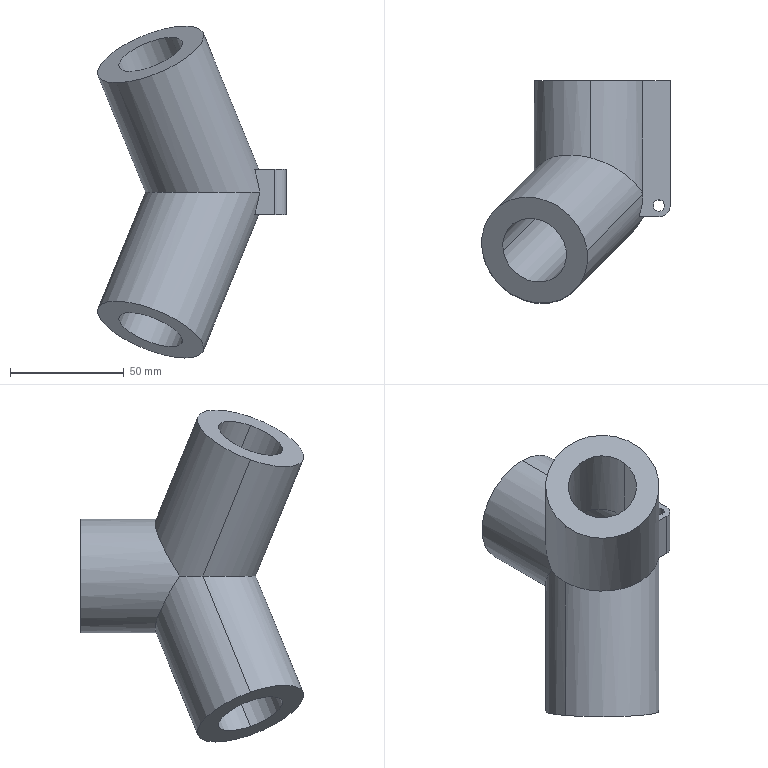Part | SolidWorks | features Cut 5, ICE 4, 3DProfileFeature 2, Fillet 1, RefAxis 1, Sweep 1 | 1 solid | 30 faces | box 83.134 x 98.134 x 146.244 mm | volume 202808 mm3 | cylinder 16 | plane 14 | commonest cylinder face diameters 50 x7 30 x4 5 x2 40 x2 10 x1
STEP:
#1=CARTESIAN_POINT('',(27.5,-5.,-10.));
#2=VERTEX_POINT('',#1);
#3=CARTESIAN_POINT('',(32.5,-5.,-10.));
#4=VERTEX_POINT('',#3);
#5=CARTESIAN_POINT('',(30.,-5.,-10.));
#6=DIRECTION('',(0.,0.,1.));
#7=DIRECTION('',(0.,-1.,0.));
#8=AXIS2_PLACEMENT_3D('',#5,#6,#7);
#9=CIRCLE('',#8,2.5);
#10=EDGE_CURVE('',#2,#4,#9,.T.);
#11=ORIENTED_EDGE('',*,*,#10,.F.);
#12=CARTESIAN_POINT('',(27.5,-5.,10.));
#13=VERTEX_POINT('',#12);
#14=CARTESIAN_POINT('',(27.5,-5.,-73.122));
#15=DIRECTION('',(0.,0.,1.));
#16=VECTOR('',#15,1000.);
#17=LINE('',#14,#16);
#18=EDGE_CURVE('',#2,#13,#17,.T.);
#19=ORIENTED_EDGE('',*,*,#18,.T.);
#20=CARTESIAN_POINT('',(32.5,-5.,10.));
#21=VERTEX_POINT('',#20);
#22=CARTESIAN_POINT('',(30.,-5.,10.));
#23=DIRECTION('',(0.,0.,-1.));
#24=DIRECTION('',(0.,1.,0.));
#25=AXIS2_PLACEMENT_3D('',#22,#23,#24);
#26=CIRCLE('',#25,2.5);
#27=EDGE_CURVE('',#21,#13,#26,.T.);
#28=ORIENTED_EDGE('',*,*,#27,.F.);
#29=CARTESIAN_POINT('',(32.5,-5.,-73.122));
#30=DIRECTION('',(0.,0.,1.));
#31=VECTOR('',#30,1000.);
#32=LINE('',#29,#31);
#33=EDGE_CURVE('',#4,#21,#32,.T.);
#34=ORIENTED_EDGE('',*,*,#33,.F.);
#35=EDGE_LOOP('',(#11,#19,#28,#34));
#36=FACE_OUTER_BOUND('',#35,.T.);
#37=CARTESIAN_POINT('',(30.,-5.,-73.122));
#38=DIRECTION('',(0.,0.,1.));
#39=DIRECTION('',(1.,0.,0.));
#40=AXIS2_PLACEMENT_3D('',#37,#38,#39);
#41=CYLINDRICAL_SURFACE('',#40,2.5);
#42=ADVANCED_FACE('',(#36),#41,.F.);
#43=CARTESIAN_POINT('',(0.,6.852,-20.));
#44=VERTEX_POINT('',#43);
#45=CARTESIAN_POINT('',(-18.438,0.,-7.748));
#46=VERTEX_POINT('',#45);
#47=CARTESIAN_POINT('',(0.,6.852,-20.));
#48=CARTESIAN_POINT('',(-1.016,7.294,-20.));
#49=CARTESIAN_POINT('',(-2.058,7.647,-19.923));
#50=CARTESIAN_POINT('',(-3.657,8.046,-19.67));
#51=CARTESIAN_POINT('',(-4.198,8.157,-19.562));
#52=CARTESIAN_POINT('',(-5.263,8.33,-19.303));
#53=CARTESIAN_POINT('',(-5.791,8.392,-19.151));
#54=CARTESIAN_POINT('',(-6.834,8.468,-18.804));
#55=CARTESIAN_POINT('',(-7.351,8.483,-18.608));
#56=CARTESIAN_POINT('',(-8.373,8.464,-18.172));
#57=CARTESIAN_POINT('',(-8.88,8.43,-17.929));
#58=CARTESIAN_POINT('',(-10.344,8.256,-17.153));
#59=CARTESIAN_POINT('',(-11.257,8.047,-16.566));
#60=CARTESIAN_POINT('',(-12.538,7.591,-15.591));
#61=CARTESIAN_POINT('',(-12.949,7.415,-15.251));
#62=CARTESIAN_POINT('',(-13.723,7.024,-14.559));
#63=CARTESIAN_POINT('',(-14.088,6.807,-14.205));
#64=CARTESIAN_POINT('',(-14.78,6.331,-13.483));
#65=CARTESIAN_POINT('',(-15.106,6.072,-13.116));
#66=CARTESIAN_POINT('',(-15.72,5.507,-12.374));
#67=CARTESIAN_POINT('',(-16.006,5.204,-12.001));
#68=CARTESIAN_POINT('',(-16.793,4.24,-10.901));
#69=CARTESIAN_POINT('',(-17.23,3.522,-10.184));
#70=CARTESIAN_POINT('',(-17.773,2.297,-9.179));
#71=CARTESIAN_POINT('',(-17.935,1.866,-8.858));
#72=CARTESIAN_POINT('',(-18.215,0.9656,-8.265));
#73=CARTESIAN_POINT('',(-18.336,0.4948,-7.992));
#74=CARTESIAN_POINT('',(-18.438,0.,-7.748));
#75=B_SPLINE_CURVE_WITH_KNOTS('',3,(#47,#48,#49,#50,#51,#52,#53,#54,#55,#56,#57,#58,#59,#60,#61,#62,#63,#64,#65,#66,#67,#68,#69,#70,#71,#72,#73,#74),.UNSPECIFIED.,.F.,.F.,(4,2,2,2,2,2,2,2,2,2,2,2,2,4),(0.01062,0.01393,0.01559,0.01724,0.0189,0.02055,0.02386,0.02551,0.02717,0.02882,0.03048,0.03379,0.03544,0.0371),.UNSPECIFIED.);
#76=EDGE_CURVE('',#44,#46,#75,.T.);
#77=ORIENTED_EDGE('',*,*,#76,.F.);
#78=CARTESIAN_POINT('',(0.,50.,-20.));
#79=VERTEX_POINT('',#78);
#80=CARTESIAN_POINT('',(0.,0.,-20.));
#81=DIRECTION('',(0.,1.,0.));
#82=VECTOR('',#81,1000.);
#83=LINE('',#80,#82);
#84=EDGE_CURVE('',#44,#79,#83,.T.);
#85=ORIENTED_EDGE('',*,*,#84,.T.);
#86=CARTESIAN_POINT('',(0.,50.,20.));
#87=VERTEX_POINT('',#86);
#88=CARTESIAN_POINT('',(0.,50.,0.));
#89=DIRECTION('',(0.,1.,0.));
#90=DIRECTION('',(0.,0.,1.));
#91=AXIS2_PLACEMENT_3D('',#88,#89,#90);
#92=CIRCLE('',#91,20.);
#93=EDGE_CURVE('',#79,#87,#92,.T.);
#94=ORIENTED_EDGE('',*,*,#93,.T.);
#95=CARTESIAN_POINT('',(0.,6.852,20.));
#96=VERTEX_POINT('',#95);
#97=CARTESIAN_POINT('',(0.,0.,20.));
#98=DIRECTION('',(0.,1.,0.));
#99=VECTOR('',#98,1000.);
#100=LINE('',#97,#99);
#101=EDGE_CURVE('',#96,#87,#100,.T.);
#102=ORIENTED_EDGE('',*,*,#101,.F.);
#103=CARTESIAN_POINT('',(-18.438,0.,7.748));
#104=VERTEX_POINT('',#103);
#105=CARTESIAN_POINT('',(-18.438,0.,7.748));
#106=CARTESIAN_POINT('',(-18.233,0.9913,8.236));
#107=CARTESIAN_POINT('',(-17.958,1.877,8.836));
#108=CARTESIAN_POINT('',(-17.421,3.093,9.831));
#109=CARTESIAN_POINT('',(-17.22,3.48,10.181));
#110=CARTESIAN_POINT('',(-16.776,4.213,10.898));
#111=CARTESIAN_POINT('',(-16.534,4.556,11.262));
#112=CARTESIAN_POINT('',(-16.01,5.199,11.996));
#113=CARTESIAN_POINT('',(-15.727,5.5,12.365));
#114=CARTESIAN_POINT('',(-15.117,6.062,13.104));
#115=CARTESIAN_POINT('',(-14.788,6.325,13.475));
#116=CARTESIAN_POINT('',(-13.744,7.045,14.564));
#117=CARTESIAN_POINT('',(-12.977,7.433,15.256));
#118=CARTESIAN_POINT('',(-11.919,7.812,16.063));
#119=CARTESIAN_POINT('',(-11.702,7.882,16.221));
#120=CARTESIAN_POINT('',(-11.259,8.011,16.532));
#121=CARTESIAN_POINT('',(-11.031,8.071,16.685));
#122=CARTESIAN_POINT('',(-10.339,8.23,17.129));
#123=CARTESIAN_POINT('',(-9.865,8.312,17.406));
#124=CARTESIAN_POINT('',(-8.896,8.428,17.921));
#125=CARTESIAN_POINT('',(-8.399,8.463,18.159));
#126=CARTESIAN_POINT('',(-7.383,8.483,18.596));
#127=CARTESIAN_POINT('',(-6.861,8.47,18.795));
#128=CARTESIAN_POINT('',(-5.273,8.355,19.325));
#129=CARTESIAN_POINT('',(-4.21,8.183,19.581));
#130=CARTESIAN_POINT('',(-2.614,7.786,19.836));
#131=CARTESIAN_POINT('',(-2.078,7.629,19.899));
#132=CARTESIAN_POINT('',(-1.025,7.272,19.981));
#133=CARTESIAN_POINT('',(-0.5076,7.073,20.));
#134=CARTESIAN_POINT('',(0.,6.852,20.));
#135=B_SPLINE_CURVE_WITH_KNOTS('',3,(#105,#106,#107,#108,#109,#110,#111,#112,#113,#114,#115,#116,#117,#118,#119,#120,#121,#122,#123,#124,#125,#126,#127,#128,#129,#130,#131,#132,#133,#134),.UNSPECIFIED.,.F.,.F.,(4,2,2,2,2,2,2,2,2,2,2,2,2,2,4),(0.,0.003311,0.004967,0.006622,0.008278,0.009933,0.01324,0.01407,0.0149,0.01656,0.01821,0.01987,0.02318,0.02483,0.02649),.UNSPECIFIED.);
#136=EDGE_CURVE('',#104,#96,#135,.T.);
#137=ORIENTED_EDGE('',*,*,#136,.F.);
#138=CARTESIAN_POINT('',(0.,0.,0.));
#139=DIRECTION('',(0.,1.,0.));
#140=DIRECTION('',(0.,0.,1.));
#141=AXIS2_PLACEMENT_3D('',#138,#139,#140);
#142=CIRCLE('',#141,20.);
#143=EDGE_CURVE('',#46,#104,#142,.T.);
#144=ORIENTED_EDGE('',*,*,#143,.F.);
#145=EDGE_LOOP('',(#77,#85,#94,#102,#137,#144));
#146=FACE_OUTER_BOUND('',#145,.T.);
#147=CARTESIAN_POINT('',(0.,0.,0.));
#148=DIRECTION('',(0.,1.,0.));
#149=DIRECTION('',(0.,0.,1.));
#150=AXIS2_PLACEMENT_3D('',#147,#148,#149);
#151=CYLINDRICAL_SURFACE('',#150,20.);
#152=ADVANCED_FACE('',(#146),#151,.F.);
#153=CARTESIAN_POINT('',(10.352,-3.536,-14.33));
#154=VERTEX_POINT('',#153);
#155=CARTESIAN_POINT('',(-17.423,-3.536,-2.991));
#156=VERTEX_POINT('',#155);
#157=CARTESIAN_POINT('',(-3.536,-3.536,-8.66));
#158=DIRECTION('',(-0.3536,-0.3536,-0.866));
#159=DIRECTION('',(-0.9258,0.,0.378));
#160=AXIS2_PLACEMENT_3D('',#157,#158,#159);
#161=CIRCLE('',#160,15.);
#162=EDGE_CURVE('',#154,#156,#161,.T.);
#163=ORIENTED_EDGE('',*,*,#162,.F.);
#164=CARTESIAN_POINT('',(-10.861,-24.749,-66.291));
#165=VERTEX_POINT('',#164);
#166=CARTESIAN_POINT('',(10.352,-3.536,-14.33));
#167=DIRECTION('',(-0.3536,-0.3536,-0.866));
#168=VECTOR('',#167,1000.);
#169=LINE('',#166,#168);
#170=EDGE_CURVE('',#154,#165,#169,.T.);
#171=ORIENTED_EDGE('',*,*,#170,.T.);
#172=CARTESIAN_POINT('',(-38.636,-24.749,-54.952));
#173=VERTEX_POINT('',#172);
#174=CARTESIAN_POINT('',(-24.749,-24.749,-60.622));
#175=DIRECTION('',(-0.3536,-0.3536,-0.866));
#176=DIRECTION('',(-0.9258,0.,0.378));
#177=AXIS2_PLACEMENT_3D('',#174,#175,#176);
#178=CIRCLE('',#177,15.);
#179=EDGE_CURVE('',#165,#173,#178,.T.);
#180=ORIENTED_EDGE('',*,*,#179,.T.);
#181=CARTESIAN_POINT('',(-17.423,-3.536,-2.991));
#182=DIRECTION('',(-0.3536,-0.3536,-0.866));
#183=VECTOR('',#182,1000.);
#184=LINE('',#181,#183);
#185=EDGE_CURVE('',#156,#173,#184,.T.);
#186=ORIENTED_EDGE('',*,*,#185,.F.);
#187=EDGE_LOOP('',(#163,#171,#180,#186));
#188=FACE_OUTER_BOUND('',#187,.T.);
#189=CARTESIAN_POINT('',(-3.536,-3.536,-8.66));
#190=DIRECTION('',(-0.3536,-0.3536,-0.866));
#191=DIRECTION('',(-0.9258,0.,0.378));
#192=AXIS2_PLACEMENT_3D('',#189,#190,#191);
#193=CYLINDRICAL_SURFACE('',#192,15.);
#194=ADVANCED_FACE('',(#188),#193,.F.);
#195=CARTESIAN_POINT('',(-17.423,-3.536,2.991));
#196=VERTEX_POINT('',#195);
#197=CARTESIAN_POINT('',(10.352,-3.536,14.33));
#198=VERTEX_POINT('',#197);
#199=CARTESIAN_POINT('',(-3.536,-3.536,8.66));
#200=DIRECTION('',(-0.3536,-0.3536,0.866));
#201=DIRECTION('',(0.9258,0.,0.378));
#202=AXIS2_PLACEMENT_3D('',#199,#200,#201);
#203=CIRCLE('',#202,15.);
#204=EDGE_CURVE('',#196,#198,#203,.T.);
#205=ORIENTED_EDGE('',*,*,#204,.F.);
#206=CARTESIAN_POINT('',(-38.636,-24.749,54.952));
#207=VERTEX_POINT('',#206);
#208=CARTESIAN_POINT('',(-17.423,-3.536,2.991));
#209=DIRECTION('',(-0.3536,-0.3536,0.866));
#210=VECTOR('',#209,1000.);
#211=LINE('',#208,#210);
#212=EDGE_CURVE('',#196,#207,#211,.T.);
#213=ORIENTED_EDGE('',*,*,#212,.T.);
#214=CARTESIAN_POINT('',(-10.861,-24.749,66.291));
#215=VERTEX_POINT('',#214);
#216=CARTESIAN_POINT('',(-24.749,-24.749,60.622));
#217=DIRECTION('',(-0.3536,-0.3536,0.866));
#218=DIRECTION('',(0.9258,0.,0.378));
#219=AXIS2_PLACEMENT_3D('',#216,#217,#218);
#220=CIRCLE('',#219,15.);
#221=EDGE_CURVE('',#207,#215,#220,.T.);
#222=ORIENTED_EDGE('',*,*,#221,.T.);
#223=CARTESIAN_POINT('',(10.352,-3.536,14.33));
#224=DIRECTION('',(-0.3536,-0.3536,0.866));
#225=VECTOR('',#224,1000.);
#226=LINE('',#223,#225);
#227=EDGE_CURVE('',#198,#215,#226,.T.);
#228=ORIENTED_EDGE('',*,*,#227,.F.);
#229=EDGE_LOOP('',(#205,#213,#222,#228));
#230=FACE_OUTER_BOUND('',#229,.T.);
#231=CARTESIAN_POINT('',(-3.536,-3.536,8.66));
#232=DIRECTION('',(-0.3536,-0.3536,0.866));
#233=DIRECTION('',(0.9258,0.,0.378));
#234=AXIS2_PLACEMENT_3D('',#231,#232,#233);
#235=CYLINDRICAL_SURFACE('',#234,15.);
#236=ADVANCED_FACE('',(#230),#235,.F.);
#237=CARTESIAN_POINT('',(0.,50.,25.));
#238=VERTEX_POINT('',#237);
#239=CARTESIAN_POINT('',(22.913,50.,10.));
#240=VERTEX_POINT('',#239);
#241=CARTESIAN_POINT('',(0.,50.,0.));
#242=DIRECTION('',(0.,1.,0.));
#243=DIRECTION('',(0.,0.,1.));
#244=AXIS2_PLACEMENT_3D('',#241,#242,#243);
#245=CIRCLE('',#244,25.);
#246=EDGE_CURVE('',#238,#240,#245,.T.);
#247=ORIENTED_EDGE('',*,*,#246,.F.);
#248=CARTESIAN_POINT('',(0.,15.995,25.));
#249=VERTEX_POINT('',#248);
#250=CARTESIAN_POINT('',(0.,50.,25.));
#251=DIRECTION('',(0.,-1.,0.));
#252=VECTOR('',#251,1000.);
#253=LINE('',#250,#252);
#254=EDGE_CURVE('',#238,#249,#253,.T.);
#255=ORIENTED_EDGE('',*,*,#254,.T.);
#256=CARTESIAN_POINT('',(22.913,0.4132,10.));
#257=VERTEX_POINT('',#256);
#258=CARTESIAN_POINT('',(0.,15.995,25.));
#259=CARTESIAN_POINT('',(10.244,13.32,25.));
#260=CARTESIAN_POINT('',(18.815,7.491,19.389));
#261=CARTESIAN_POINT('',(22.913,0.4132,10.));
#262=(BOUNDED_CURVE()B_SPLINE_CURVE(3,(#258,#259,#260,#261),.UNSPECIFIED.,.F.,.F.)B_SPLINE_CURVE_WITH_KNOTS((4,4),(3.529,4.688),.UNSPECIFIED.)CURVE()GEOMETRIC_REPRESENTATION_ITEM()RATIONAL_B_SPLINE_CURVE((1.,0.8911,0.8911,1.))REPRESENTATION_ITEM(''));
#263=EDGE_CURVE('',#249,#257,#262,.T.);
#264=ORIENTED_EDGE('',*,*,#263,.T.);
#265=CARTESIAN_POINT('',(22.913,50.,10.));
#266=DIRECTION('',(0.,-1.,0.));
#267=VECTOR('',#266,1000.);
#268=LINE('',#265,#267);
#269=EDGE_CURVE('',#240,#257,#268,.T.);
#270=ORIENTED_EDGE('',*,*,#269,.F.);
#271=EDGE_LOOP('',(#247,#255,#264,#270));
#272=FACE_OUTER_BOUND('',#271,.T.);
#273=CARTESIAN_POINT('',(0.,50.,0.));
#274=DIRECTION('',(0.,-1.,0.));
#275=DIRECTION('',(0.,0.,-1.));
#276=AXIS2_PLACEMENT_3D('',#273,#274,#275);
#277=CYLINDRICAL_SURFACE('',#276,25.);
#278=ADVANCED_FACE('',(#272),#277,.T.);
#279=ORIENTED_EDGE('',*,*,#254,.F.);
#280=CARTESIAN_POINT('',(0.,50.,-25.));
#281=VERTEX_POINT('',#280);
#282=CARTESIAN_POINT('',(0.,50.,0.));
#283=DIRECTION('',(0.,1.,0.));
#284=DIRECTION('',(0.,0.,1.));
#285=AXIS2_PLACEMENT_3D('',#282,#283,#284);
#286=CIRCLE('',#285,25.);
#287=EDGE_CURVE('',#281,#238,#286,.T.);
#288=ORIENTED_EDGE('',*,*,#287,.F.);
#289=CARTESIAN_POINT('',(0.,15.995,-25.));
#290=VERTEX_POINT('',#289);
#291=CARTESIAN_POINT('',(0.,50.,-25.));
#292=DIRECTION('',(0.,-1.,0.));
#293=VECTOR('',#292,1000.);
#294=LINE('',#291,#293);
#295=EDGE_CURVE('',#281,#290,#294,.T.);
#296=ORIENTED_EDGE('',*,*,#295,.T.);
#297=CARTESIAN_POINT('',(-25.,6.53,0.));
#298=VERTEX_POINT('',#297);
#299=CARTESIAN_POINT('',(0.,15.995,-25.));
#300=CARTESIAN_POINT('',(-14.645,19.821,-25.));
#301=CARTESIAN_POINT('',(-25.,15.9,-14.645));
#302=CARTESIAN_POINT('',(-25.,6.53,0.));
#303=(BOUNDED_CURVE()B_SPLINE_CURVE(3,(#299,#300,#301,#302),.UNSPECIFIED.,.F.,.F.)B_SPLINE_CURVE_WITH_KNOTS((4,4),(5.896,7.466),.UNSPECIFIED.)CURVE()GEOMETRIC_REPRESENTATION_ITEM()RATIONAL_B_SPLINE_CURVE((1.,0.8047,0.8047,1.))REPRESENTATION_ITEM(''));
#304=EDGE_CURVE('',#290,#298,#303,.T.);
#305=ORIENTED_EDGE('',*,*,#304,.T.);
#306=CARTESIAN_POINT('',(-25.,6.53,0.));
#307=CARTESIAN_POINT('',(-25.,15.9,14.645));
#308=CARTESIAN_POINT('',(-14.645,19.821,25.));
#309=CARTESIAN_POINT('',(0.,15.995,25.));
#310=(BOUNDED_CURVE()B_SPLINE_CURVE(3,(#306,#307,#308,#309),.UNSPECIFIED.,.F.,.F.)B_SPLINE_CURVE_WITH_KNOTS((4,4),(1.958,3.529),.UNSPECIFIED.)CURVE()GEOMETRIC_REPRESENTATION_ITEM()RATIONAL_B_SPLINE_CURVE((1.,0.8047,0.8047,1.))REPRESENTATION_ITEM(''));
#311=EDGE_CURVE('',#298,#249,#310,.T.);
#312=ORIENTED_EDGE('',*,*,#311,.T.);
#313=EDGE_LOOP('',(#279,#288,#296,#305,#312));
#314=FACE_OUTER_BOUND('',#313,.T.);
#315=CARTESIAN_POINT('',(0.,50.,0.));
#316=DIRECTION('',(0.,-1.,0.));
#317=DIRECTION('',(0.,0.,-1.));
#318=AXIS2_PLACEMENT_3D('',#315,#316,#317);
#319=CYLINDRICAL_SURFACE('',#318,25.);
#320=ADVANCED_FACE('',(#314),#319,.T.);
#321=CARTESIAN_POINT('',(-1.603,-24.749,70.071));
#322=VERTEX_POINT('',#321);
#323=CARTESIAN_POINT('',(-47.894,-24.749,51.173));
#324=VERTEX_POINT('',#323);
#325=CARTESIAN_POINT('',(-24.749,-24.749,60.622));
#326=DIRECTION('',(-0.3536,-0.3536,0.866));
#327=DIRECTION('',(0.9258,0.,0.378));
#328=AXIS2_PLACEMENT_3D('',#325,#326,#327);
#329=CIRCLE('',#328,25.);
#330=EDGE_CURVE('',#322,#324,#329,.T.);
#331=ORIENTED_EDGE('',*,*,#330,.F.);
#332=CARTESIAN_POINT('',(22.921,-0.2249,10.));
#333=VERTEX_POINT('',#332);
#334=CARTESIAN_POINT('',(-1.603,-24.749,70.071));
#335=DIRECTION('',(0.3536,0.3536,-0.866));
#336=VECTOR('',#335,1000.);
#337=LINE('',#334,#336);
#338=EDGE_CURVE('',#322,#333,#337,.T.);
#339=ORIENTED_EDGE('',*,*,#338,.T.);
#340=CARTESIAN_POINT('',(22.913,0.4132,10.));
#341=CARTESIAN_POINT('',(22.918,0.2009,10.));
#342=CARTESIAN_POINT('',(22.921,-0.0118,10.));
#343=CARTESIAN_POINT('',(22.921,-0.2249,10.));
#344=(BOUNDED_CURVE()B_SPLINE_CURVE(3,(#340,#341,#342,#343),.UNSPECIFIED.,.F.,.F.)B_SPLINE_CURVE_WITH_KNOTS((4,4),(0.6898,0.7137),.UNSPECIFIED.)CURVE()GEOMETRIC_REPRESENTATION_ITEM()RATIONAL_B_SPLINE_CURVE((1.,1.,1.,1.))REPRESENTATION_ITEM(''));
#345=EDGE_CURVE('',#257,#333,#344,.T.);
#346=ORIENTED_EDGE('',*,*,#345,.F.);
#347=ORIENTED_EDGE('',*,*,#263,.F.);
#348=ORIENTED_EDGE('',*,*,#311,.F.);
#349=CARTESIAN_POINT('',(-27.003,-3.858,0.));
#350=VERTEX_POINT('',#349);
#351=CARTESIAN_POINT('',(-27.003,-3.858,0.));
#352=CARTESIAN_POINT('',(-27.003,-0.3828,0.));
#353=CARTESIAN_POINT('',(-26.327,3.124,0.));
#354=CARTESIAN_POINT('',(-25.,6.53,0.));
#355=(BOUNDED_CURVE()B_SPLINE_CURVE(3,(#351,#352,#353,#354),.UNSPECIFIED.,.F.,.F.)B_SPLINE_CURVE_WITH_KNOTS((4,4),(3.855,4.243),.UNSPECIFIED.)CURVE()GEOMETRIC_REPRESENTATION_ITEM()RATIONAL_B_SPLINE_CURVE((1.,0.9875,0.9875,1.))REPRESENTATION_ITEM(''));
#356=EDGE_CURVE('',#350,#298,#355,.T.);
#357=ORIENTED_EDGE('',*,*,#356,.F.);
#358=CARTESIAN_POINT('',(-47.894,-24.749,51.173));
#359=DIRECTION('',(0.3536,0.3536,-0.866));
#360=VECTOR('',#359,1000.);
#361=LINE('',#358,#360);
#362=EDGE_CURVE('',#324,#350,#361,.T.);
#363=ORIENTED_EDGE('',*,*,#362,.F.);
#364=EDGE_LOOP('',(#331,#339,#346,#347,#348,#357,#363));
#365=FACE_OUTER_BOUND('',#364,.T.);
#366=CARTESIAN_POINT('',(-24.749,-24.749,60.622));
#367=DIRECTION('',(0.3536,0.3536,-0.866));
#368=DIRECTION('',(-0.9258,0.,-0.378));
#369=AXIS2_PLACEMENT_3D('',#366,#367,#368);
#370=CYLINDRICAL_SURFACE('',#369,25.);
#371=ADVANCED_FACE('',(#365),#370,.T.);
#372=CARTESIAN_POINT('',(22.921,-0.2249,-10.));
#373=VERTEX_POINT('',#372);
#374=CARTESIAN_POINT('',(22.913,0.4132,-10.));
#375=VERTEX_POINT('',#374);
#376=CARTESIAN_POINT('',(22.921,-0.2249,-10.));
#377=CARTESIAN_POINT('',(22.921,-0.0118,-10.));
#378=CARTESIAN_POINT('',(22.918,0.2009,-10.));
#379=CARTESIAN_POINT('',(22.913,0.4132,-10.));
#380=(BOUNDED_CURVE()B_SPLINE_CURVE(3,(#376,#377,#378,#379),.UNSPECIFIED.,.F.,.T.)B_SPLINE_CURVE_WITH_KNOTS((4,4),(2.428,2.452),.UNSPECIFIED.)CURVE()GEOMETRIC_REPRESENTATION_ITEM()RATIONAL_B_SPLINE_CURVE((1.,1.,1.,1.))REPRESENTATION_ITEM(''));
#381=EDGE_CURVE('',#373,#375,#380,.T.);
#382=ORIENTED_EDGE('',*,*,#381,.F.);
#383=CARTESIAN_POINT('',(-1.603,-24.749,-70.071));
#384=VERTEX_POINT('',#383);
#385=CARTESIAN_POINT('',(34.774,11.628,19.034));
#386=DIRECTION('',(-0.3536,-0.3536,-0.866));
#387=VECTOR('',#386,1000.);
#388=LINE('',#385,#387);
#389=EDGE_CURVE('',#373,#384,#388,.T.);
#390=ORIENTED_EDGE('',*,*,#389,.T.);
#391=CARTESIAN_POINT('',(-47.894,-24.749,-51.173));
#392=VERTEX_POINT('',#391);
#393=CARTESIAN_POINT('',(-24.749,-24.749,-60.622));
#394=DIRECTION('',(0.3536,0.3536,0.866));
#395=DIRECTION('',(0.9258,0.,-0.378));
#396=AXIS2_PLACEMENT_3D('',#393,#394,#395);
#397=CIRCLE('',#396,25.);
#398=EDGE_CURVE('',#384,#392,#397,.T.);
#399=ORIENTED_EDGE('',*,*,#398,.T.);
#400=CARTESIAN_POINT('',(-11.517,11.628,37.933));
#401=DIRECTION('',(-0.3536,-0.3536,-0.866));
#402=VECTOR('',#401,1000.);
#403=LINE('',#400,#402);
#404=EDGE_CURVE('',#350,#392,#403,.T.);
#405=ORIENTED_EDGE('',*,*,#404,.F.);
#406=ORIENTED_EDGE('',*,*,#356,.T.);
#407=ORIENTED_EDGE('',*,*,#304,.F.);
#408=CARTESIAN_POINT('',(22.913,0.4132,-10.));
#409=CARTESIAN_POINT('',(18.815,7.491,-19.389));
#410=CARTESIAN_POINT('',(10.244,13.32,-25.));
#411=CARTESIAN_POINT('',(0.,15.995,-25.));
#412=(BOUNDED_CURVE()B_SPLINE_CURVE(3,(#408,#409,#410,#411),.UNSPECIFIED.,.F.,.F.)B_SPLINE_CURVE_WITH_KNOTS((4,4),(4.736,5.896),.UNSPECIFIED.)CURVE()GEOMETRIC_REPRESENTATION_ITEM()RATIONAL_B_SPLINE_CURVE((1.,0.8911,0.8911,1.))REPRESENTATION_ITEM(''));
#413=EDGE_CURVE('',#375,#290,#412,.T.);
#414=ORIENTED_EDGE('',*,*,#413,.F.);
#415=EDGE_LOOP('',(#382,#390,#399,#405,#406,#407,#414));
#416=FACE_OUTER_BOUND('',#415,.T.);
#417=CARTESIAN_POINT('',(11.628,11.628,28.484));
#418=DIRECTION('',(-0.3536,-0.3536,-0.866));
#419=DIRECTION('',(-0.9258,0.,0.378));
#420=AXIS2_PLACEMENT_3D('',#417,#418,#419);
#421=CYLINDRICAL_SURFACE('',#420,25.);
#422=ADVANCED_FACE('',(#416),#421,.T.);
#423=ORIENTED_EDGE('',*,*,#389,.F.);
#424=CARTESIAN_POINT('',(21.149,-10.,-10.));
#425=VERTEX_POINT('',#424);
#426=CARTESIAN_POINT('',(21.149,-10.,-10.));
#427=CARTESIAN_POINT('',(22.323,-6.783,-10.));
#428=CARTESIAN_POINT('',(22.921,-3.488,-10.));
#429=CARTESIAN_POINT('',(22.921,-0.2249,-10.));
#430=(BOUNDED_CURVE()B_SPLINE_CURVE(3,(#426,#427,#428,#429),.UNSPECIFIED.,.F.,.F.)B_SPLINE_CURVE_WITH_KNOTS((4,4),(2.064,2.428),.UNSPECIFIED.)CURVE()GEOMETRIC_REPRESENTATION_ITEM()RATIONAL_B_SPLINE_CURVE((1.,0.989,0.989,1.))REPRESENTATION_ITEM(''));
#431=EDGE_CURVE('',#425,#373,#430,.T.);
#432=ORIENTED_EDGE('',*,*,#431,.F.);
#433=CARTESIAN_POINT('',(23.397,-10.,0.));
#434=VERTEX_POINT('',#433);
#435=CARTESIAN_POINT('',(23.397,-10.,0.));
#436=CARTESIAN_POINT('',(22.784,-10.,-3.248));
#437=CARTESIAN_POINT('',(22.033,-10.,-6.588));
#438=CARTESIAN_POINT('',(21.149,-10.,-10.));
#439=(BOUNDED_CURVE()B_SPLINE_CURVE(3,(#435,#436,#437,#438),.UNSPECIFIED.,.F.,.F.)B_SPLINE_CURVE_WITH_KNOTS((4,4),(4.19,4.348),.UNSPECIFIED.)CURVE()GEOMETRIC_REPRESENTATION_ITEM()RATIONAL_B_SPLINE_CURVE((1.,0.9979,0.9979,1.))REPRESENTATION_ITEM(''));
#440=EDGE_CURVE('',#434,#425,#439,.T.);
#441=ORIENTED_EDGE('',*,*,#440,.F.);
#442=CARTESIAN_POINT('',(23.397,-10.,0.));
#443=CARTESIAN_POINT('',(6.226,-41.951,0.));
#444=CARTESIAN_POINT('',(-27.003,-37.901,0.));
#445=CARTESIAN_POINT('',(-27.003,-3.858,0.));
#446=(BOUNDED_CURVE()B_SPLINE_CURVE(3,(#442,#443,#444,#445),.UNSPECIFIED.,.F.,.F.)B_SPLINE_CURVE_WITH_KNOTS((4,4),(1.236,3.855),.UNSPECIFIED.)CURVE()GEOMETRIC_REPRESENTATION_ITEM()RATIONAL_B_SPLINE_CURVE((1.,0.5056,0.5056,1.))REPRESENTATION_ITEM(''));
#447=EDGE_CURVE('',#434,#350,#446,.T.);
#448=ORIENTED_EDGE('',*,*,#447,.T.);
#449=ORIENTED_EDGE('',*,*,#404,.T.);
#450=CARTESIAN_POINT('',(-24.749,-24.749,-60.622));
#451=DIRECTION('',(0.3536,0.3536,0.866));
#452=DIRECTION('',(0.9258,0.,-0.378));
#453=AXIS2_PLACEMENT_3D('',#450,#451,#452);
#454=CIRCLE('',#453,25.);
#455=EDGE_CURVE('',#392,#384,#454,.T.);
#456=ORIENTED_EDGE('',*,*,#455,.T.);
#457=EDGE_LOOP('',(#423,#432,#441,#448,#449,#456));
#458=FACE_OUTER_BOUND('',#457,.T.);
#459=CARTESIAN_POINT('',(11.628,11.628,28.484));
#460=DIRECTION('',(-0.3536,-0.3536,-0.866));
#461=DIRECTION('',(-0.9258,0.,0.378));
#462=AXIS2_PLACEMENT_3D('',#459,#460,#461);
#463=CYLINDRICAL_SURFACE('',#462,25.);
#464=ADVANCED_FACE('',(#458),#463,.T.);
#465=ORIENTED_EDGE('',*,*,#338,.F.);
#466=CARTESIAN_POINT('',(-24.749,-24.749,60.622));
#467=DIRECTION('',(-0.3536,-0.3536,0.866));
#468=DIRECTION('',(0.9258,0.,0.378));
#469=AXIS2_PLACEMENT_3D('',#466,#467,#468);
#470=CIRCLE('',#469,25.);
#471=EDGE_CURVE('',#324,#322,#470,.T.);
#472=ORIENTED_EDGE('',*,*,#471,.F.);
#473=ORIENTED_EDGE('',*,*,#362,.T.);
#474=ORIENTED_EDGE('',*,*,#447,.F.);
#475=CARTESIAN_POINT('',(21.149,-10.,10.));
#476=VERTEX_POINT('',#475);
#477=CARTESIAN_POINT('',(21.149,-10.,10.));
#478=CARTESIAN_POINT('',(22.033,-10.,6.588));
#479=CARTESIAN_POINT('',(22.784,-10.,3.248));
#480=CARTESIAN_POINT('',(23.397,-10.,0.));
#481=(BOUNDED_CURVE()B_SPLINE_CURVE(3,(#477,#478,#479,#480),.UNSPECIFIED.,.F.,.F.)B_SPLINE_CURVE_WITH_KNOTS((4,4),(5.077,5.235),.UNSPECIFIED.)CURVE()GEOMETRIC_REPRESENTATION_ITEM()RATIONAL_B_SPLINE_CURVE((1.,0.9979,0.9979,1.))REPRESENTATION_ITEM(''));
#482=EDGE_CURVE('',#476,#434,#481,.T.);
#483=ORIENTED_EDGE('',*,*,#482,.F.);
#484=CARTESIAN_POINT('',(22.921,-0.2249,10.));
#485=CARTESIAN_POINT('',(22.921,-3.488,10.));
#486=CARTESIAN_POINT('',(22.323,-6.783,10.));
#487=CARTESIAN_POINT('',(21.149,-10.,10.));
#488=(BOUNDED_CURVE()B_SPLINE_CURVE(3,(#484,#485,#486,#487),.UNSPECIFIED.,.F.,.F.)B_SPLINE_CURVE_WITH_KNOTS((4,4),(0.7137,1.078),.UNSPECIFIED.)CURVE()GEOMETRIC_REPRESENTATION_ITEM()RATIONAL_B_SPLINE_CURVE((1.,0.989,0.989,1.))REPRESENTATION_ITEM(''));
#489=EDGE_CURVE('',#333,#476,#488,.T.);
#490=ORIENTED_EDGE('',*,*,#489,.F.);
#491=EDGE_LOOP('',(#465,#472,#473,#474,#483,#490));
#492=FACE_OUTER_BOUND('',#491,.T.);
#493=CARTESIAN_POINT('',(-24.749,-24.749,60.622));
#494=DIRECTION('',(0.3536,0.3536,-0.866));
#495=DIRECTION('',(-0.9258,0.,-0.378));
#496=AXIS2_PLACEMENT_3D('',#493,#494,#495);
#497=CYLINDRICAL_SURFACE('',#496,25.);
#498=ADVANCED_FACE('',(#492),#497,.T.);
#499=ORIENTED_EDGE('',*,*,#295,.F.);
#500=CARTESIAN_POINT('',(22.913,50.,-10.));
#501=VERTEX_POINT('',#500);
#502=CARTESIAN_POINT('',(0.,50.,0.));
#503=DIRECTION('',(0.,1.,0.));
#504=DIRECTION('',(0.,0.,1.));
#505=AXIS2_PLACEMENT_3D('',#502,#503,#504);
#506=CIRCLE('',#505,25.);
#507=EDGE_CURVE('',#501,#281,#506,.T.);
#508=ORIENTED_EDGE('',*,*,#507,.F.);
#509=CARTESIAN_POINT('',(22.913,50.,-10.));
#510=DIRECTION('',(0.,1.,0.));
#511=VECTOR('',#510,1000.);
#512=LINE('',#509,#511);
#513=EDGE_CURVE('',#375,#501,#512,.T.);
#514=ORIENTED_EDGE('',*,*,#513,.F.);
#515=ORIENTED_EDGE('',*,*,#413,.T.);
#516=EDGE_LOOP('',(#499,#508,#514,#515));
#517=FACE_OUTER_BOUND('',#516,.T.);
#518=CARTESIAN_POINT('',(0.,50.,0.));
#519=DIRECTION('',(0.,-1.,0.));
#520=DIRECTION('',(0.,0.,-1.));
#521=AXIS2_PLACEMENT_3D('',#518,#519,#520);
#522=CYLINDRICAL_SURFACE('',#521,25.);
#523=ADVANCED_FACE('',(#517),#522,.T.);
#524=ORIENTED_EDGE('',*,*,#212,.F.);
#525=CARTESIAN_POINT('',(-17.48,0.,4.411));
#526=VERTEX_POINT('',#525);
#527=CARTESIAN_POINT('',(-3.536,-3.536,8.66));
#528=DIRECTION('',(-0.3536,-0.3536,0.866));
#529=DIRECTION('',(0.9258,0.,0.378));
#530=AXIS2_PLACEMENT_3D('',#527,#528,#529);
#531=CIRCLE('',#530,15.);
#532=EDGE_CURVE('',#526,#196,#531,.T.);
#533=ORIENTED_EDGE('',*,*,#532,.F.);
#534=CARTESIAN_POINT('',(-18.438,0.,7.748));
#535=CARTESIAN_POINT('',(-18.141,0.,6.643));
#536=CARTESIAN_POINT('',(-17.821,0.,5.53));
#537=CARTESIAN_POINT('',(-17.48,0.,4.411));
#538=(BOUNDED_CURVE()B_SPLINE_CURVE(3,(#534,#535,#536,#537),.UNSPECIFIED.,.F.,.F.)B_SPLINE_CURVE_WITH_KNOTS((4,4),(1.231,1.316),.UNSPECIFIED.)CURVE()GEOMETRIC_REPRESENTATION_ITEM()RATIONAL_B_SPLINE_CURVE((1.,0.9994,0.9994,1.))REPRESENTATION_ITEM(''));
#539=EDGE_CURVE('',#104,#526,#538,.T.);
#540=ORIENTED_EDGE('',*,*,#539,.F.);
#541=ORIENTED_EDGE('',*,*,#136,.T.);
#542=CARTESIAN_POINT('',(7.748,0.,18.438));
#543=VERTEX_POINT('',#542);
#544=CARTESIAN_POINT('',(0.,6.852,20.));
#545=CARTESIAN_POINT('',(0.8132,6.499,20.));
#546=CARTESIAN_POINT('',(1.603,6.091,19.95));
#547=CARTESIAN_POINT('',(3.124,5.158,19.769));
#548=CARTESIAN_POINT('',(3.837,4.645,19.64));
#549=CARTESIAN_POINT('',(4.831,3.796,19.411));
#550=CARTESIAN_POINT('',(5.15,3.5,19.328));
#551=CARTESIAN_POINT('',(5.761,2.877,19.155));
#552=CARTESIAN_POINT('',(6.054,2.549,19.064));
#553=CARTESIAN_POINT('',(6.881,1.525,18.788));
#554=CARTESIAN_POINT('',(7.357,0.7932,18.603));
#555=CARTESIAN_POINT('',(7.748,0.,18.438));
#556=B_SPLINE_CURVE_WITH_KNOTS('',3,(#544,#545,#546,#547,#548,#549,#550,#551,#552,#553,#554,#555),.UNSPECIFIED.,.F.,.F.,(4,2,2,2,2,4),(0.02649,0.02914,0.03179,0.03312,0.03445,0.0371),.UNSPECIFIED.);
#557=EDGE_CURVE('',#96,#543,#556,.T.);
#558=ORIENTED_EDGE('',*,*,#557,.T.);
#559=CARTESIAN_POINT('',(9.399,0.,15.384));
#560=VERTEX_POINT('',#559);
#561=CARTESIAN_POINT('',(9.399,0.,15.384));
#562=CARTESIAN_POINT('',(8.859,0.,16.422));
#563=CARTESIAN_POINT('',(8.308,0.,17.441));
#564=CARTESIAN_POINT('',(7.748,0.,18.438));
#565=(BOUNDED_CURVE()B_SPLINE_CURVE(3,(#561,#562,#563,#564),.UNSPECIFIED.,.F.,.F.)B_SPLINE_CURVE_WITH_KNOTS((4,4),(4.967,5.052),.UNSPECIFIED.)CURVE()GEOMETRIC_REPRESENTATION_ITEM()RATIONAL_B_SPLINE_CURVE((1.,0.9994,0.9994,1.))REPRESENTATION_ITEM(''));
#566=EDGE_CURVE('',#560,#543,#565,.T.);
#567=ORIENTED_EDGE('',*,*,#566,.F.);
#568=CARTESIAN_POINT('',(-3.536,-3.536,8.66));
#569=DIRECTION('',(-0.3536,-0.3536,0.866));
#570=DIRECTION('',(0.9258,0.,0.378));
#571=AXIS2_PLACEMENT_3D('',#568,#569,#570);
#572=CIRCLE('',#571,15.);
#573=EDGE_CURVE('',#198,#560,#572,.T.);
#574=ORIENTED_EDGE('',*,*,#573,.F.);
#575=ORIENTED_EDGE('',*,*,#227,.T.);
#576=CARTESIAN_POINT('',(-24.749,-24.749,60.622));
#577=DIRECTION('',(-0.3536,-0.3536,0.866));
#578=DIRECTION('',(0.9258,0.,0.378));
#579=AXIS2_PLACEMENT_3D('',#576,#577,#578);
#580=CIRCLE('',#579,15.);
#581=EDGE_CURVE('',#215,#207,#580,.T.);
#582=ORIENTED_EDGE('',*,*,#581,.T.);
#583=EDGE_LOOP('',(#524,#533,#540,#541,#558,#567,#574,#575,#582));
#584=FACE_OUTER_BOUND('',#583,.T.);
#585=CARTESIAN_POINT('',(-3.536,-3.536,8.66));
#586=DIRECTION('',(-0.3536,-0.3536,0.866));
#587=DIRECTION('',(0.9258,0.,0.378));
#588=AXIS2_PLACEMENT_3D('',#585,#586,#587);
#589=CYLINDRICAL_SURFACE('',#588,15.);
#590=ADVANCED_FACE('',(#584),#589,.F.);
#591=ORIENTED_EDGE('',*,*,#532,.T.);
#592=ORIENTED_EDGE('',*,*,#204,.T.);
#593=ORIENTED_EDGE('',*,*,#573,.T.);
#594=CARTESIAN_POINT('',(-4.041,0.,9.897));
#595=DIRECTION('',(-0.9258,0.,-0.378));
#596=VECTOR('',#595,1000.);
#597=LINE('',#594,#596);
#598=EDGE_CURVE('',#560,#526,#597,.T.);
#599=ORIENTED_EDGE('',*,*,#598,.T.);
#600=EDGE_LOOP('',(#591,#592,#593,#599));
#601=FACE_OUTER_BOUND('',#600,.T.);
#602=CARTESIAN_POINT('',(-3.536,-3.536,8.66));
#603=DIRECTION('',(-0.3536,-0.3536,0.866));
#604=DIRECTION('',(0.9258,0.,0.378));
#605=AXIS2_PLACEMENT_3D('',#602,#603,#604);
#606=PLANE('',#605);
#607=ADVANCED_FACE('',(#601),#606,.T.);
#608=ORIENTED_EDGE('',*,*,#170,.F.);
#609=CARTESIAN_POINT('',(9.399,0.,-15.384));
#610=VERTEX_POINT('',#609);
#611=CARTESIAN_POINT('',(-3.536,-3.536,-8.66));
#612=DIRECTION('',(-0.3536,-0.3536,-0.866));
#613=DIRECTION('',(-0.9258,0.,0.378));
#614=AXIS2_PLACEMENT_3D('',#611,#612,#613);
#615=CIRCLE('',#614,15.);
#616=EDGE_CURVE('',#610,#154,#615,.T.);
#617=ORIENTED_EDGE('',*,*,#616,.F.);
#618=CARTESIAN_POINT('',(7.748,0.,-18.438));
#619=VERTEX_POINT('',#618);
#620=CARTESIAN_POINT('',(7.748,0.,-18.438));
#621=CARTESIAN_POINT('',(8.308,0.,-17.441));
#622=CARTESIAN_POINT('',(8.859,0.,-16.422));
#623=CARTESIAN_POINT('',(9.399,0.,-15.384));
#624=(BOUNDED_CURVE()B_SPLINE_CURVE(3,(#620,#621,#622,#623),.UNSPECIFIED.,.F.,.F.)B_SPLINE_CURVE_WITH_KNOTS((4,4),(1.231,1.316),.UNSPECIFIED.)CURVE()GEOMETRIC_REPRESENTATION_ITEM()RATIONAL_B_SPLINE_CURVE((1.,0.9994,0.9994,1.))REPRESENTATION_ITEM(''));
#625=EDGE_CURVE('',#619,#610,#624,.T.);
#626=ORIENTED_EDGE('',*,*,#625,.F.);
#627=CARTESIAN_POINT('',(7.748,0.,-18.438));
#628=CARTESIAN_POINT('',(7.356,0.7949,-18.603));
#629=CARTESIAN_POINT('',(6.882,1.522,-18.787));
#630=CARTESIAN_POINT('',(6.067,2.535,-19.06));
#631=CARTESIAN_POINT('',(5.778,2.859,-19.15));
#632=CARTESIAN_POINT('',(5.166,3.484,-19.324));
#633=CARTESIAN_POINT('',(4.842,3.786,-19.408));
#634=CARTESIAN_POINT('',(3.839,4.644,-19.64));
#635=CARTESIAN_POINT('',(3.125,5.157,-19.769));
#636=CARTESIAN_POINT('',(1.994,5.851,-19.904));
#637=CARTESIAN_POINT('',(1.607,6.07,-19.939));
#638=CARTESIAN_POINT('',(0.8118,6.483,-19.987));
#639=CARTESIAN_POINT('',(0.4075,6.675,-20.));
#640=CARTESIAN_POINT('',(0.,6.852,-20.));
#641=B_SPLINE_CURVE_WITH_KNOTS('',3,(#627,#628,#629,#630,#631,#632,#633,#634,#635,#636,#637,#638,#639,#640),.UNSPECIFIED.,.F.,.F.,(4,2,2,2,2,2,4),(0.,0.002655,0.003983,0.005311,0.007966,0.009293,0.01062),.UNSPECIFIED.);
#642=EDGE_CURVE('',#619,#44,#641,.T.);
#643=ORIENTED_EDGE('',*,*,#642,.T.);
#644=ORIENTED_EDGE('',*,*,#76,.T.);
#645=CARTESIAN_POINT('',(-17.48,0.,-4.411));
#646=VERTEX_POINT('',#645);
#647=CARTESIAN_POINT('',(-17.48,0.,-4.411));
#648=CARTESIAN_POINT('',(-17.821,0.,-5.53));
#649=CARTESIAN_POINT('',(-18.141,0.,-6.643));
#650=CARTESIAN_POINT('',(-18.438,0.,-7.748));
#651=(BOUNDED_CURVE()B_SPLINE_CURVE(3,(#647,#648,#649,#650),.UNSPECIFIED.,.F.,.T.)B_SPLINE_CURVE_WITH_KNOTS((4,4),(4.967,5.052),.UNSPECIFIED.)CURVE()GEOMETRIC_REPRESENTATION_ITEM()RATIONAL_B_SPLINE_CURVE((1.,0.9994,0.9994,1.))REPRESENTATION_ITEM(''));
#652=EDGE_CURVE('',#646,#46,#651,.T.);
#653=ORIENTED_EDGE('',*,*,#652,.F.);
#654=CARTESIAN_POINT('',(-3.536,-3.536,-8.66));
#655=DIRECTION('',(-0.3536,-0.3536,-0.866));
#656=DIRECTION('',(-0.9258,0.,0.378));
#657=AXIS2_PLACEMENT_3D('',#654,#655,#656);
#658=CIRCLE('',#657,15.);
#659=EDGE_CURVE('',#156,#646,#658,.T.);
#660=ORIENTED_EDGE('',*,*,#659,.F.);
#661=ORIENTED_EDGE('',*,*,#185,.T.);
#662=CARTESIAN_POINT('',(-24.749,-24.749,-60.622));
#663=DIRECTION('',(-0.3536,-0.3536,-0.866));
#664=DIRECTION('',(-0.9258,0.,0.378));
#665=AXIS2_PLACEMENT_3D('',#662,#663,#664);
#666=CIRCLE('',#665,15.);
#667=EDGE_CURVE('',#173,#165,#666,.T.);
#668=ORIENTED_EDGE('',*,*,#667,.T.);
#669=EDGE_LOOP('',(#608,#617,#626,#643,#644,#653,#660,#661,#668));
#670=FACE_OUTER_BOUND('',#669,.T.);
#671=CARTESIAN_POINT('',(-3.536,-3.536,-8.66));
#672=DIRECTION('',(-0.3536,-0.3536,-0.866));
#673=DIRECTION('',(-0.9258,0.,0.378));
#674=AXIS2_PLACEMENT_3D('',#671,#672,#673);
#675=CYLINDRICAL_SURFACE('',#674,15.);
#676=ADVANCED_FACE('',(#670),#675,.F.);
#677=ORIENTED_EDGE('',*,*,#616,.T.);
#678=ORIENTED_EDGE('',*,*,#162,.T.);
#679=ORIENTED_EDGE('',*,*,#659,.T.);
#680=CARTESIAN_POINT('',(-4.041,0.,-9.897));
#681=DIRECTION('',(0.9258,0.,-0.378));
#682=VECTOR('',#681,1000.);
#683=LINE('',#680,#682);
#684=EDGE_CURVE('',#646,#610,#683,.T.);
#685=ORIENTED_EDGE('',*,*,#684,.T.);
#686=EDGE_LOOP('',(#677,#678,#679,#685));
#687=FACE_OUTER_BOUND('',#686,.T.);
#688=CARTESIAN_POINT('',(-3.536,-3.536,-8.66));
#689=DIRECTION('',(-0.3536,-0.3536,-0.866));
#690=DIRECTION('',(-0.9258,0.,0.378));
#691=AXIS2_PLACEMENT_3D('',#688,#689,#690);
#692=PLANE('',#691);
#693=ADVANCED_FACE('',(#687),#692,.T.);
#694=ORIENTED_EDGE('',*,*,#581,.F.);
#695=ORIENTED_EDGE('',*,*,#221,.F.);
#696=EDGE_LOOP('',(#694,#695));
#697=FACE_BOUND('',#696,.T.);
#698=ORIENTED_EDGE('',*,*,#471,.T.);
#699=ORIENTED_EDGE('',*,*,#330,.T.);
#700=EDGE_LOOP('',(#698,#699));
#701=FACE_OUTER_BOUND('',#700,.T.);
#702=CARTESIAN_POINT('',(-24.749,-24.749,60.622));
#703=DIRECTION('',(-0.3536,-0.3536,0.866));
#704=DIRECTION('',(0.9258,0.,0.378));
#705=AXIS2_PLACEMENT_3D('',#702,#703,#704);
#706=PLANE('',#705);
#707=ADVANCED_FACE('',(#697,#701),#706,.T.);
#708=ORIENTED_EDGE('',*,*,#667,.F.);
#709=ORIENTED_EDGE('',*,*,#179,.F.);
#710=EDGE_LOOP('',(#708,#709));
#711=FACE_BOUND('',#710,.T.);
#712=ORIENTED_EDGE('',*,*,#455,.F.);
#713=ORIENTED_EDGE('',*,*,#398,.F.);
#714=EDGE_LOOP('',(#712,#713));
#715=FACE_OUTER_BOUND('',#714,.T.);
#716=CARTESIAN_POINT('',(-24.749,-24.749,-60.622));
#717=DIRECTION('',(0.3536,0.3536,0.866));
#718=DIRECTION('',(0.9258,0.,-0.378));
#719=AXIS2_PLACEMENT_3D('',#716,#717,#718);
#720=PLANE('',#719);
#721=ADVANCED_FACE('',(#711,#715),#720,.F.);
#722=CARTESIAN_POINT('',(35.,50.,-1.));
#723=VERTEX_POINT('',#722);
#724=CARTESIAN_POINT('',(29.998,50.,-1.));
#725=VERTEX_POINT('',#724);
#726=CARTESIAN_POINT('',(29.998,50.,-1.));
#727=DIRECTION('',(-1.,0.,0.));
#728=VECTOR('',#727,1000.);
#729=LINE('',#726,#728);
#730=EDGE_CURVE('',#723,#725,#729,.T.);
#731=ORIENTED_EDGE('',*,*,#730,.F.);
#732=CARTESIAN_POINT('',(35.,50.,-10.));
#733=VERTEX_POINT('',#732);
#734=CARTESIAN_POINT('',(35.,50.,10.));
#735=DIRECTION('',(0.,0.,1.));
#736=VECTOR('',#735,1000.);
#737=LINE('',#734,#736);
#738=EDGE_CURVE('',#733,#723,#737,.T.);
#739=ORIENTED_EDGE('',*,*,#738,.F.);
#740=CARTESIAN_POINT('',(35.,50.,-10.));
#741=DIRECTION('',(-1.,0.,0.));
#742=VECTOR('',#741,1000.);
#743=LINE('',#740,#742);
#744=EDGE_CURVE('',#733,#501,#743,.T.);
#745=ORIENTED_EDGE('',*,*,#744,.T.);
#746=ORIENTED_EDGE('',*,*,#507,.T.);
#747=ORIENTED_EDGE('',*,*,#287,.T.);
#748=ORIENTED_EDGE('',*,*,#246,.T.);
#749=CARTESIAN_POINT('',(35.,50.,10.));
#750=VERTEX_POINT('',#749);
#751=CARTESIAN_POINT('',(35.,50.,10.));
#752=DIRECTION('',(-1.,0.,0.));
#753=VECTOR('',#752,1000.);
#754=LINE('',#751,#753);
#755=EDGE_CURVE('',#750,#240,#754,.T.);
#756=ORIENTED_EDGE('',*,*,#755,.F.);
#757=CARTESIAN_POINT('',(35.,50.,1.));
#758=VERTEX_POINT('',#757);
#759=CARTESIAN_POINT('',(35.,50.,10.));
#760=DIRECTION('',(0.,0.,1.));
#761=VECTOR('',#760,1000.);
#762=LINE('',#759,#761);
#763=EDGE_CURVE('',#758,#750,#762,.T.);
#764=ORIENTED_EDGE('',*,*,#763,.F.);
#765=CARTESIAN_POINT('',(29.998,50.,1.));
#766=VERTEX_POINT('',#765);
#767=CARTESIAN_POINT('',(35.,50.,1.));
#768=DIRECTION('',(1.,0.,0.));
#769=VECTOR('',#768,1000.);
#770=LINE('',#767,#769);
#771=EDGE_CURVE('',#766,#758,#770,.T.);
#772=ORIENTED_EDGE('',*,*,#771,.F.);
#773=CARTESIAN_POINT('',(29.998,50.,1.));
#774=DIRECTION('',(0.,0.,1.));
#775=VECTOR('',#774,1000.);
#776=LINE('',#773,#775);
#777=EDGE_CURVE('',#725,#766,#776,.T.);
#778=ORIENTED_EDGE('',*,*,#777,.F.);
#779=EDGE_LOOP('',(#731,#739,#745,#746,#747,#748,#756,#764,#772,#778));
#780=FACE_OUTER_BOUND('',#779,.T.);
#781=CARTESIAN_POINT('',(0.,50.,0.));
#782=DIRECTION('',(0.,1.,0.));
#783=DIRECTION('',(0.,0.,1.));
#784=AXIS2_PLACEMENT_3D('',#781,#782,#783);
#785=CIRCLE('',#784,20.);
#786=EDGE_CURVE('',#87,#79,#785,.T.);
#787=ORIENTED_EDGE('',*,*,#786,.F.);
#788=ORIENTED_EDGE('',*,*,#93,.F.);
#789=EDGE_LOOP('',(#787,#788));
#790=FACE_BOUND('',#789,.T.);
#791=CARTESIAN_POINT('',(0.,50.,0.));
#792=DIRECTION('',(0.,1.,0.));
#793=DIRECTION('',(0.,0.,1.));
#794=AXIS2_PLACEMENT_3D('',#791,#792,#793);
#795=PLANE('',#794);
#796=ADVANCED_FACE('',(#780,#790),#795,.T.);
#797=ORIENTED_EDGE('',*,*,#84,.F.);
#798=ORIENTED_EDGE('',*,*,#642,.F.);
#799=CARTESIAN_POINT('',(0.,0.,0.));
#800=DIRECTION('',(0.,1.,0.));
#801=DIRECTION('',(0.,0.,1.));
#802=AXIS2_PLACEMENT_3D('',#799,#800,#801);
#803=CIRCLE('',#802,20.);
#804=EDGE_CURVE('',#543,#619,#803,.T.);
#805=ORIENTED_EDGE('',*,*,#804,.F.);
#806=ORIENTED_EDGE('',*,*,#557,.F.);
#807=ORIENTED_EDGE('',*,*,#101,.T.);
#808=ORIENTED_EDGE('',*,*,#786,.T.);
#809=EDGE_LOOP('',(#797,#798,#805,#806,#807,#808));
#810=FACE_OUTER_BOUND('',#809,.T.);
#811=CARTESIAN_POINT('',(0.,0.,0.));
#812=DIRECTION('',(0.,1.,0.));
#813=DIRECTION('',(0.,0.,1.));
#814=AXIS2_PLACEMENT_3D('',#811,#812,#813);
#815=CYLINDRICAL_SURFACE('',#814,20.);
#816=ADVANCED_FACE('',(#810),#815,.F.);
#817=ORIENTED_EDGE('',*,*,#539,.T.);
#818=ORIENTED_EDGE('',*,*,#598,.F.);
#819=ORIENTED_EDGE('',*,*,#566,.T.);
#820=ORIENTED_EDGE('',*,*,#804,.T.);
#821=ORIENTED_EDGE('',*,*,#625,.T.);
#822=ORIENTED_EDGE('',*,*,#684,.F.);
#823=ORIENTED_EDGE('',*,*,#652,.T.);
#824=ORIENTED_EDGE('',*,*,#143,.T.);
#825=EDGE_LOOP('',(#817,#818,#819,#820,#821,#822,#823,#824));
#826=FACE_OUTER_BOUND('',#825,.T.);
#827=CARTESIAN_POINT('',(0.,0.,0.));
#828=DIRECTION('',(0.,1.,0.));
#829=DIRECTION('',(0.,0.,1.));
#830=AXIS2_PLACEMENT_3D('',#827,#828,#829);
#831=PLANE('',#830);
#832=ADVANCED_FACE('',(#826),#831,.T.);
#833=CARTESIAN_POINT('',(30.,-5.,-10.));
#834=DIRECTION('',(0.,0.,1.));
#835=DIRECTION('',(0.,-1.,0.));
#836=AXIS2_PLACEMENT_3D('',#833,#834,#835);
#837=CIRCLE('',#836,2.5);
#838=EDGE_CURVE('',#4,#2,#837,.T.);
#839=ORIENTED_EDGE('',*,*,#838,.T.);
#840=ORIENTED_EDGE('',*,*,#10,.T.);
#841=EDGE_LOOP('',(#839,#840));
#842=FACE_BOUND('',#841,.T.);
#843=CARTESIAN_POINT('',(35.,-5.,-10.));
#844=VERTEX_POINT('',#843);
#845=CARTESIAN_POINT('',(35.,-10.,-10.));
#846=DIRECTION('',(0.,1.,0.));
#847=VECTOR('',#846,1000.);
#848=LINE('',#845,#847);
#849=EDGE_CURVE('',#844,#733,#848,.T.);
#850=ORIENTED_EDGE('',*,*,#849,.F.);
#851=CARTESIAN_POINT('',(30.,-10.,-10.));
#852=VERTEX_POINT('',#851);
#853=CARTESIAN_POINT('',(30.,-5.,-10.));
#854=DIRECTION('',(0.,0.,-1.));
#855=DIRECTION('',(0.,-1.,0.));
#856=AXIS2_PLACEMENT_3D('',#853,#854,#855);
#857=CIRCLE('',#856,5.);
#858=EDGE_CURVE('',#844,#852,#857,.T.);
#859=ORIENTED_EDGE('',*,*,#858,.T.);
#860=CARTESIAN_POINT('',(35.,-10.,-10.));
#861=DIRECTION('',(-1.,0.,0.));
#862=VECTOR('',#861,1000.);
#863=LINE('',#860,#862);
#864=EDGE_CURVE('',#852,#425,#863,.T.);
#865=ORIENTED_EDGE('',*,*,#864,.T.);
#866=ORIENTED_EDGE('',*,*,#431,.T.);
#867=ORIENTED_EDGE('',*,*,#381,.T.);
#868=ORIENTED_EDGE('',*,*,#513,.T.);
#869=ORIENTED_EDGE('',*,*,#744,.F.);
#870=EDGE_LOOP('',(#850,#859,#865,#866,#867,#868,#869));
#871=FACE_OUTER_BOUND('',#870,.T.);
#872=CARTESIAN_POINT('',(35.,-10.,-10.));
#873=DIRECTION('',(0.,0.,1.));
#874=DIRECTION('',(0.,-1.,0.));
#875=AXIS2_PLACEMENT_3D('',#872,#873,#874);
#876=PLANE('',#875);
#877=ADVANCED_FACE('',(#842,#871),#876,.F.);
#878=ORIENTED_EDGE('',*,*,#27,.T.);
#879=CARTESIAN_POINT('',(30.,-5.,10.));
#880=DIRECTION('',(0.,0.,-1.));
#881=DIRECTION('',(0.,1.,0.));
#882=AXIS2_PLACEMENT_3D('',#879,#880,#881);
#883=CIRCLE('',#882,2.5);
#884=EDGE_CURVE('',#13,#21,#883,.T.);
#885=ORIENTED_EDGE('',*,*,#884,.T.);
#886=EDGE_LOOP('',(#878,#885));
#887=FACE_BOUND('',#886,.T.);
#888=CARTESIAN_POINT('',(30.,-10.,10.));
#889=VERTEX_POINT('',#888);
#890=CARTESIAN_POINT('',(35.,-10.,10.));
#891=DIRECTION('',(-1.,0.,0.));
#892=VECTOR('',#891,1000.);
#893=LINE('',#890,#892);
#894=EDGE_CURVE('',#889,#476,#893,.T.);
#895=ORIENTED_EDGE('',*,*,#894,.F.);
#896=CARTESIAN_POINT('',(35.,-5.,10.));
#897=VERTEX_POINT('',#896);
#898=CARTESIAN_POINT('',(30.,-5.,10.));
#899=DIRECTION('',(0.,0.,1.));
#900=DIRECTION('',(0.,1.,0.));
#901=AXIS2_PLACEMENT_3D('',#898,#899,#900);
#902=CIRCLE('',#901,5.);
#903=EDGE_CURVE('',#889,#897,#902,.T.);
#904=ORIENTED_EDGE('',*,*,#903,.T.);
#905=CARTESIAN_POINT('',(35.,-10.,10.));
#906=DIRECTION('',(0.,-1.,0.));
#907=VECTOR('',#906,1000.);
#908=LINE('',#905,#907);
#909=EDGE_CURVE('',#750,#897,#908,.T.);
#910=ORIENTED_EDGE('',*,*,#909,.F.);
#911=ORIENTED_EDGE('',*,*,#755,.T.);
#912=ORIENTED_EDGE('',*,*,#269,.T.);
#913=ORIENTED_EDGE('',*,*,#345,.T.);
#914=ORIENTED_EDGE('',*,*,#489,.T.);
#915=EDGE_LOOP('',(#895,#904,#910,#911,#912,#913,#914));
#916=FACE_OUTER_BOUND('',#915,.T.);
#917=CARTESIAN_POINT('',(35.,-10.,10.));
#918=DIRECTION('',(0.,0.,-1.));
#919=DIRECTION('',(0.,1.,0.));
#920=AXIS2_PLACEMENT_3D('',#917,#918,#919);
#921=PLANE('',#920);
#922=ADVANCED_FACE('',(#887,#916),#921,.F.);
#923=ORIENTED_EDGE('',*,*,#864,.F.);
#924=CARTESIAN_POINT('',(30.,-10.,10.));
#925=DIRECTION('',(0.,0.,1.));
#926=VECTOR('',#925,1000.);
#927=LINE('',#924,#926);
#928=EDGE_CURVE('',#852,#889,#927,.T.);
#929=ORIENTED_EDGE('',*,*,#928,.T.);
#930=ORIENTED_EDGE('',*,*,#894,.T.);
#931=ORIENTED_EDGE('',*,*,#482,.T.);
#932=ORIENTED_EDGE('',*,*,#440,.T.);
#933=EDGE_LOOP('',(#923,#929,#930,#931,#932));
#934=FACE_OUTER_BOUND('',#933,.T.);
#935=CARTESIAN_POINT('',(35.,-10.,10.));
#936=DIRECTION('',(0.,1.,0.));
#937=DIRECTION('',(0.,0.,1.));
#938=AXIS2_PLACEMENT_3D('',#935,#936,#937);
#939=PLANE('',#938);
#940=ADVANCED_FACE('',(#934),#939,.F.);
#941=ORIENTED_EDGE('',*,*,#738,.T.);
#942=CARTESIAN_POINT('',(35.,20.353,-1.));
#943=VERTEX_POINT('',#942);
#944=CARTESIAN_POINT('',(35.,14.966,-1.));
#945=DIRECTION('',(0.,1.,0.));
#946=VECTOR('',#945,1000.);
#947=LINE('',#944,#946);
#948=EDGE_CURVE('',#943,#723,#947,.T.);
#949=ORIENTED_EDGE('',*,*,#948,.F.);
#950=CARTESIAN_POINT('',(35.,20.353,1.));
#951=VERTEX_POINT('',#950);
#952=CARTESIAN_POINT('',(35.,20.353,-1.));
#953=DIRECTION('',(0.,0.,-1.));
#954=VECTOR('',#953,1000.);
#955=LINE('',#952,#954);
#956=EDGE_CURVE('',#951,#943,#955,.T.);
#957=ORIENTED_EDGE('',*,*,#956,.F.);
#958=CARTESIAN_POINT('',(35.,14.966,1.));
#959=DIRECTION('',(0.,1.,0.));
#960=VECTOR('',#959,1000.);
#961=LINE('',#958,#960);
#962=EDGE_CURVE('',#951,#758,#961,.T.);
#963=ORIENTED_EDGE('',*,*,#962,.T.);
#964=ORIENTED_EDGE('',*,*,#763,.T.);
#965=ORIENTED_EDGE('',*,*,#909,.T.);
#966=CARTESIAN_POINT('',(35.,-5.,0.));
#967=DIRECTION('',(0.,0.,-1.));
#968=VECTOR('',#967,1000.);
#969=LINE('',#966,#968);
#970=EDGE_CURVE('',#897,#844,#969,.T.);
#971=ORIENTED_EDGE('',*,*,#970,.T.);
#972=ORIENTED_EDGE('',*,*,#849,.T.);
#973=EDGE_LOOP('',(#941,#949,#957,#963,#964,#965,#971,#972));
#974=FACE_OUTER_BOUND('',#973,.T.);
#975=CARTESIAN_POINT('',(35.,0.,0.));
#976=DIRECTION('',(-1.,0.,0.));
#977=DIRECTION('',(0.,0.,1.));
#978=AXIS2_PLACEMENT_3D('',#975,#976,#977);
#979=PLANE('',#978);
#980=ADVANCED_FACE('',(#974),#979,.F.);
#981=ORIENTED_EDGE('',*,*,#903,.F.);
#982=ORIENTED_EDGE('',*,*,#928,.F.);
#983=ORIENTED_EDGE('',*,*,#858,.F.);
#984=ORIENTED_EDGE('',*,*,#970,.F.);
#985=EDGE_LOOP('',(#981,#982,#983,#984));
#986=FACE_OUTER_BOUND('',#985,.T.);
#987=CARTESIAN_POINT('',(30.,-5.,0.));
#988=DIRECTION('',(0.,0.,-1.));
#989=DIRECTION('',(-1.,0.,0.));
#990=AXIS2_PLACEMENT_3D('',#987,#988,#989);
#991=CYLINDRICAL_SURFACE('',#990,5.);
#992=ADVANCED_FACE('',(#986),#991,.T.);
#993=ORIENTED_EDGE('',*,*,#18,.F.);
#994=ORIENTED_EDGE('',*,*,#838,.F.);
#995=ORIENTED_EDGE('',*,*,#33,.T.);
#996=ORIENTED_EDGE('',*,*,#884,.F.);
#997=EDGE_LOOP('',(#993,#994,#995,#996));
#998=FACE_OUTER_BOUND('',#997,.T.);
#999=CARTESIAN_POINT('',(30.,-5.,-73.122));
#1000=DIRECTION('',(0.,0.,1.));
#1001=DIRECTION('',(1.,0.,0.));
#1002=AXIS2_PLACEMENT_3D('',#999,#1000,#1001);
#1003=CYLINDRICAL_SURFACE('',#1002,2.5);
#1004=ADVANCED_FACE('',(#998),#1003,.F.);
#1005=ORIENTED_EDGE('',*,*,#948,.T.);
#1006=ORIENTED_EDGE('',*,*,#730,.T.);
#1007=CARTESIAN_POINT('',(29.998,20.353,-1.));
#1008=VERTEX_POINT('',#1007);
#1009=CARTESIAN_POINT('',(29.998,14.966,-1.));
#1010=DIRECTION('',(0.,1.,0.));
#1011=VECTOR('',#1010,1000.);
#1012=LINE('',#1009,#1011);
#1013=EDGE_CURVE('',#1008,#725,#1012,.T.);
#1014=ORIENTED_EDGE('',*,*,#1013,.F.);
#1015=CARTESIAN_POINT('',(29.998,20.353,-1.));
#1016=DIRECTION('',(-1.,0.,0.));
#1017=VECTOR('',#1016,1000.);
#1018=LINE('',#1015,#1017);
#1019=EDGE_CURVE('',#943,#1008,#1018,.T.);
#1020=ORIENTED_EDGE('',*,*,#1019,.F.);
#1021=EDGE_LOOP('',(#1005,#1006,#1014,#1020));
#1022=FACE_OUTER_BOUND('',#1021,.T.);
#1023=CARTESIAN_POINT('',(29.998,14.966,-1.));
#1024=DIRECTION('',(0.,0.,-1.));
#1025=DIRECTION('',(-1.,0.,0.));
#1026=AXIS2_PLACEMENT_3D('',#1023,#1024,#1025);
#1027=PLANE('',#1026);
#1028=ADVANCED_FACE('',(#1022),#1027,.F.);
#1029=ORIENTED_EDGE('',*,*,#1013,.T.);
#1030=ORIENTED_EDGE('',*,*,#777,.T.);
#1031=CARTESIAN_POINT('',(29.998,20.353,1.));
#1032=VERTEX_POINT('',#1031);
#1033=CARTESIAN_POINT('',(29.998,14.966,1.));
#1034=DIRECTION('',(0.,1.,0.));
#1035=VECTOR('',#1034,1000.);
#1036=LINE('',#1033,#1035);
#1037=EDGE_CURVE('',#1032,#766,#1036,.T.);
#1038=ORIENTED_EDGE('',*,*,#1037,.F.);
#1039=CARTESIAN_POINT('',(29.998,20.353,-1.));
#1040=DIRECTION('',(0.,0.,1.));
#1041=VECTOR('',#1040,1000.);
#1042=LINE('',#1039,#1041);
#1043=EDGE_CURVE('',#1008,#1032,#1042,.T.);
#1044=ORIENTED_EDGE('',*,*,#1043,.F.);
#1045=EDGE_LOOP('',(#1029,#1030,#1038,#1044));
#1046=FACE_OUTER_BOUND('',#1045,.T.);
#1047=CARTESIAN_POINT('',(29.998,14.966,1.));
#1048=DIRECTION('',(-1.,0.,0.));
#1049=DIRECTION('',(0.,0.,1.));
#1050=AXIS2_PLACEMENT_3D('',#1047,#1048,#1049);
#1051=PLANE('',#1050);
#1052=ADVANCED_FACE('',(#1046),#1051,.F.);
#1053=ORIENTED_EDGE('',*,*,#1037,.T.);
#1054=ORIENTED_EDGE('',*,*,#771,.T.);
#1055=ORIENTED_EDGE('',*,*,#962,.F.);
#1056=CARTESIAN_POINT('',(814.479,20.353,1.));
#1057=DIRECTION('',(1.,0.,0.));
#1058=VECTOR('',#1057,1000.);
#1059=LINE('',#1056,#1058);
#1060=EDGE_CURVE('',#1032,#951,#1059,.T.);
#1061=ORIENTED_EDGE('',*,*,#1060,.F.);
#1062=EDGE_LOOP('',(#1053,#1054,#1055,#1061));
#1063=FACE_OUTER_BOUND('',#1062,.T.);
#1064=CARTESIAN_POINT('',(35.,14.966,1.));
#1065=DIRECTION('',(0.,0.,1.));
#1066=DIRECTION('',(1.,0.,0.));
#1067=AXIS2_PLACEMENT_3D('',#1064,#1065,#1066);
#1068=PLANE('',#1067);
#1069=ADVANCED_FACE('',(#1063),#1068,.F.);
#1070=ORIENTED_EDGE('',*,*,#956,.T.);
#1071=ORIENTED_EDGE('',*,*,#1019,.T.);
#1072=ORIENTED_EDGE('',*,*,#1043,.T.);
#1073=ORIENTED_EDGE('',*,*,#1060,.T.);
#1074=EDGE_LOOP('',(#1070,#1071,#1072,#1073));
#1075=FACE_OUTER_BOUND('',#1074,.T.);
#1076=CARTESIAN_POINT('',(384.738,20.353,-10.));
#1077=DIRECTION('',(0.,-1.,0.));
#1078=DIRECTION('',(0.,0.,-1.));
#1079=AXIS2_PLACEMENT_3D('',#1076,#1077,#1078);
#1080=PLANE('',#1079);
#1081=ADVANCED_FACE('',(#1075),#1080,.F.);
#1082=CLOSED_SHELL('',(#42,#152,#194,#236,#278,#320,#371,#422,#464,#498,#523,#590,#607,#676,#693,#707,#721,#796,#816,#832,#877,#922,#940,#980,#992,#1004,#1028,#1052,#1069,#1081));
#1083=MANIFOLD_SOLID_BREP('',#1082);
#1084=CARTESIAN_POINT('',(0.,0.,0.));
#1085=DIRECTION('',(0.,0.,1.));
#1086=DIRECTION('',(1.,0.,0.));
#1087=AXIS2_PLACEMENT_3D('',#1084,#1085,#1086);
#1088=(LENGTH_UNIT()NAMED_UNIT(*)SI_UNIT(.MILLI.,.METRE.));
#1089=UNCERTAINTY_MEASURE_WITH_UNIT(LENGTH_MEASURE(0.00001),#1088,'','');
#1090=(NAMED_UNIT(*)PLANE_ANGLE_UNIT()SI_UNIT($,.RADIAN.));
#1091=(NAMED_UNIT(*)SI_UNIT($,.STERADIAN.)SOLID_ANGLE_UNIT());
#1092=(GEOMETRIC_REPRESENTATION_CONTEXT(3)GLOBAL_UNCERTAINTY_ASSIGNED_CONTEXT((#1089))GLOBAL_UNIT_ASSIGNED_CONTEXT((#1088,#1090,#1091))REPRESENTATION_CONTEXT('',''));
#1093=ADVANCED_BREP_SHAPE_REPRESENTATION('',(#1083,#1087),#1092);